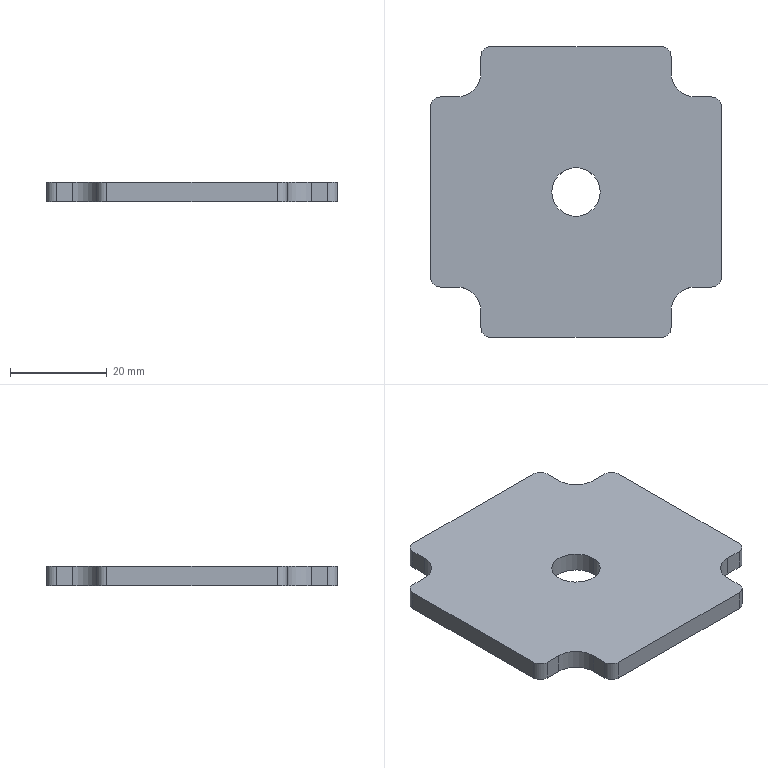Part | STEP file | 31090648--1-SOL000_1_1_1 | 1 solid | 28 faces | box 60 x 60 x 4 mm | volume 12414 mm3 | cylinder 14 | plane 14 | commonest cylinder face diameters 4 x8 10 x6